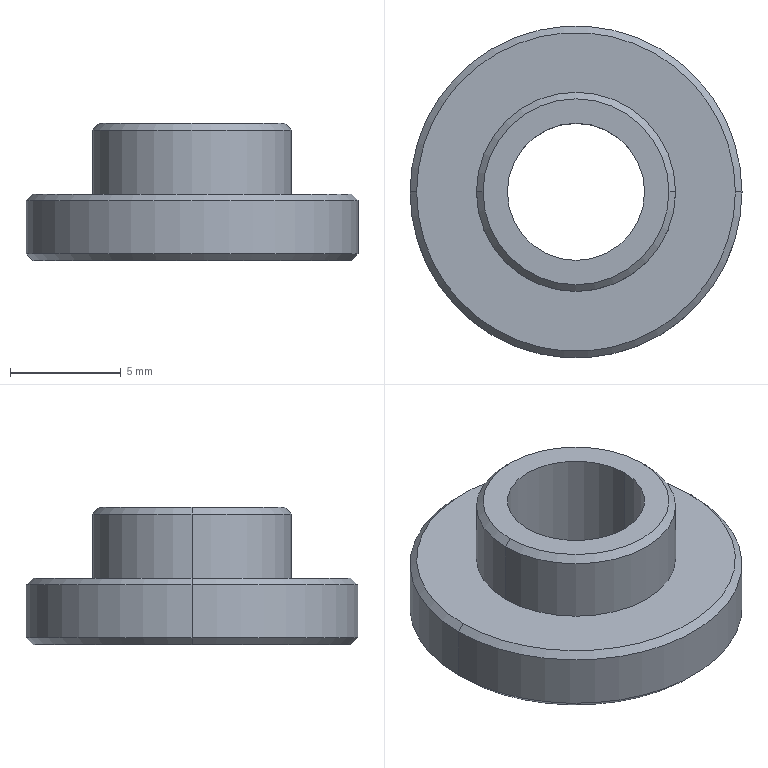Part | STEP file | Sprocket spacer | 1 solid | 15 faces | box 15 x 15 x 6.2 mm | volume 541.108 mm3 | cone 6 | cylinder 6 | plane 3 | commonest cylinder face diameters 6.2 x2 9 x2 15 x2
STEP:
#1=CARTESIAN_POINT('',(0.,0.,0.));
#2=DIRECTION('',(0.,0.,1.));
#3=DIRECTION('',(1.,0.,0.));
#4=AXIS2_PLACEMENT_3D('',#1,#2,#3);
#5=CARTESIAN_POINT('',(-7.2,0.,0.));
#6=VERTEX_POINT('',#5);
#7=CARTESIAN_POINT('',(7.2,0.,0.));
#8=VERTEX_POINT('',#7);
#9=CARTESIAN_POINT('',(0.,0.,0.));
#10=DIRECTION('',(0.,0.,-1.));
#11=DIRECTION('',(1.,0.,0.));
#12=AXIS2_PLACEMENT_3D('',#9,#10,#11);
#13=CIRCLE('',#12,7.2);
#14=CARTESIAN_POINT('',(0.,0.,0.));
#15=DIRECTION('',(0.,0.,1.));
#16=DIRECTION('',(1.,0.,0.));
#17=AXIS2_PLACEMENT_3D('',#14,#15,#16);
#18=CONICAL_SURFACE('',#17,7.2,0.7854);
#19=CARTESIAN_POINT('',(6.283,0.));
#20=DIRECTION('',(-1.,0.));
#21=VECTOR('',#20,1.);
#22=LINE('',#19,#21);
#23=(GEOMETRIC_REPRESENTATION_CONTEXT(2)PARAMETRIC_REPRESENTATION_CONTEXT()REPRESENTATION_CONTEXT('',''));
#24=DEFINITIONAL_REPRESENTATION('',(#22),#23);
#25=PCURVE('',#18,#24);
#26=CARTESIAN_POINT('',(0.,0.,0.));
#27=DIRECTION('',(0.,0.,1.));
#28=DIRECTION('',(1.,0.,0.));
#29=AXIS2_PLACEMENT_3D('',#26,#27,#28);
#30=PLANE('',#29);
#31=CARTESIAN_POINT('',(7.2,0.));
#32=CARTESIAN_POINT('',(7.2,-12.471));
#33=CARTESIAN_POINT('',(-3.6,-6.235));
#34=CARTESIAN_POINT('',(-14.4,0.));
#35=CARTESIAN_POINT('',(-3.6,6.235));
#36=CARTESIAN_POINT('',(7.2,12.471));
#37=CARTESIAN_POINT('',(7.2,0.));
#38=(BOUNDED_CURVE()B_SPLINE_CURVE(2,(#31,#32,#33,#34,#35,#36,#37),.UNSPECIFIED.,.T.,.F.)B_SPLINE_CURVE_WITH_KNOTS((1,2,2,2,2,1),(-2.094,0.,2.094,4.189,6.283,8.378),.UNSPECIFIED.)CURVE()GEOMETRIC_REPRESENTATION_ITEM()RATIONAL_B_SPLINE_CURVE((1.,0.5,1.,0.5,1.,0.5,1.))REPRESENTATION_ITEM(''));
#39=(GEOMETRIC_REPRESENTATION_CONTEXT(2)PARAMETRIC_REPRESENTATION_CONTEXT()REPRESENTATION_CONTEXT('',''));
#40=DEFINITIONAL_REPRESENTATION('',(#38),#39);
#41=PCURVE('',#30,#40);
#42=SURFACE_CURVE('',#13,(#25,#41),.PCURVE_S1.);
#43=EDGE_CURVE('',#6,#8,#42,.T.);
#44=ORIENTED_EDGE('',*,*,#43,.F.);
#45=CARTESIAN_POINT('',(-7.5,0.,0.3));
#46=VERTEX_POINT('',#45);
#47=CARTESIAN_POINT('',(-7.2,0.,0.));
#48=DIRECTION('',(-0.7071,0.,0.7071));
#49=VECTOR('',#48,1.);
#50=LINE('',#47,#49);
#51=CARTESIAN_POINT('',(3.142,0.));
#52=DIRECTION('',(0.,1.));
#53=VECTOR('',#52,1.);
#54=LINE('',#51,#53);
#55=(GEOMETRIC_REPRESENTATION_CONTEXT(2)PARAMETRIC_REPRESENTATION_CONTEXT()REPRESENTATION_CONTEXT('',''));
#56=DEFINITIONAL_REPRESENTATION('',(#54),#55);
#57=PCURVE('',#18,#56);
#58=CARTESIAN_POINT('',(0.,0.,0.));
#59=DIRECTION('',(0.,0.,1.));
#60=DIRECTION('',(1.,0.,0.));
#61=AXIS2_PLACEMENT_3D('',#58,#59,#60);
#62=CONICAL_SURFACE('',#61,7.2,0.7854);
#63=CARTESIAN_POINT('',(3.142,0.));
#64=DIRECTION('',(0.,1.));
#65=VECTOR('',#64,1.);
#66=LINE('',#63,#65);
#67=(GEOMETRIC_REPRESENTATION_CONTEXT(2)PARAMETRIC_REPRESENTATION_CONTEXT()REPRESENTATION_CONTEXT('',''));
#68=DEFINITIONAL_REPRESENTATION('',(#66),#67);
#69=PCURVE('',#62,#68);
#70=SURFACE_CURVE('',#50,(#57,#69),.PCURVE_S1.);
#71=EDGE_CURVE('',#6,#46,#70,.T.);
#72=ORIENTED_EDGE('',*,*,#71,.T.);
#73=CARTESIAN_POINT('',(7.5,0.,0.3));
#74=VERTEX_POINT('',#73);
#75=CARTESIAN_POINT('',(0.,0.,0.3));
#76=DIRECTION('',(0.,0.,1.));
#77=DIRECTION('',(1.,0.,0.));
#78=AXIS2_PLACEMENT_3D('',#75,#76,#77);
#79=CIRCLE('',#78,7.5);
#80=CARTESIAN_POINT('',(0.,0.3));
#81=DIRECTION('',(1.,0.));
#82=VECTOR('',#81,1.);
#83=LINE('',#80,#82);
#84=(GEOMETRIC_REPRESENTATION_CONTEXT(2)PARAMETRIC_REPRESENTATION_CONTEXT()REPRESENTATION_CONTEXT('',''));
#85=DEFINITIONAL_REPRESENTATION('',(#83),#84);
#86=PCURVE('',#18,#85);
#87=CARTESIAN_POINT('',(0.,0.,3.));
#88=DIRECTION('',(0.,0.,-1.));
#89=DIRECTION('',(-1.,0.,0.));
#90=AXIS2_PLACEMENT_3D('',#87,#88,#89);
#91=CYLINDRICAL_SURFACE('',#90,7.5);
#92=CARTESIAN_POINT('',(3.142,2.7));
#93=DIRECTION('',(-1.,0.));
#94=VECTOR('',#93,1.);
#95=LINE('',#92,#94);
#96=(GEOMETRIC_REPRESENTATION_CONTEXT(2)PARAMETRIC_REPRESENTATION_CONTEXT()REPRESENTATION_CONTEXT('',''));
#97=DEFINITIONAL_REPRESENTATION('',(#95),#96);
#98=PCURVE('',#91,#97);
#99=SURFACE_CURVE('',#79,(#86,#98),.PCURVE_S1.);
#100=EDGE_CURVE('',#74,#46,#99,.T.);
#101=ORIENTED_EDGE('',*,*,#100,.F.);
#102=CARTESIAN_POINT('',(7.2,0.,0.));
#103=DIRECTION('',(0.7071,0.,0.7071));
#104=VECTOR('',#103,1.);
#105=LINE('',#102,#104);
#106=CARTESIAN_POINT('',(0.,0.));
#107=DIRECTION('',(0.,1.));
#108=VECTOR('',#107,1.);
#109=LINE('',#106,#108);
#110=(GEOMETRIC_REPRESENTATION_CONTEXT(2)PARAMETRIC_REPRESENTATION_CONTEXT()REPRESENTATION_CONTEXT('',''));
#111=DEFINITIONAL_REPRESENTATION('',(#109),#110);
#112=PCURVE('',#18,#111);
#113=CARTESIAN_POINT('',(6.283,0.));
#114=DIRECTION('',(0.,1.));
#115=VECTOR('',#114,1.);
#116=LINE('',#113,#115);
#117=(GEOMETRIC_REPRESENTATION_CONTEXT(2)PARAMETRIC_REPRESENTATION_CONTEXT()REPRESENTATION_CONTEXT('',''));
#118=DEFINITIONAL_REPRESENTATION('',(#116),#117);
#119=PCURVE('',#62,#118);
#120=SURFACE_CURVE('',#105,(#112,#119),.PCURVE_S1.);
#121=EDGE_CURVE('',#8,#74,#120,.T.);
#122=ORIENTED_EDGE('',*,*,#121,.F.);
#123=EDGE_LOOP('',(#44,#72,#101,#122));
#124=FACE_BOUND('',#123,.T.);
#125=ADVANCED_FACE('',(#124),#18,.T.);
#126=CARTESIAN_POINT('',(7.2,0.,3.));
#127=VERTEX_POINT('',#126);
#128=CARTESIAN_POINT('',(-7.2,0.,3.));
#129=VERTEX_POINT('',#128);
#130=CARTESIAN_POINT('',(0.,0.,3.));
#131=DIRECTION('',(0.,0.,1.));
#132=DIRECTION('',(-1.,0.,0.));
#133=AXIS2_PLACEMENT_3D('',#130,#131,#132);
#134=CIRCLE('',#133,7.2);
#135=CARTESIAN_POINT('',(0.,0.,2.7));
#136=DIRECTION('',(0.,0.,-1.));
#137=DIRECTION('',(-1.,0.,0.));
#138=AXIS2_PLACEMENT_3D('',#135,#136,#137);
#139=CONICAL_SURFACE('',#138,7.5,0.7854);
#140=CARTESIAN_POINT('',(6.283,-0.3));
#141=DIRECTION('',(-1.,0.));
#142=VECTOR('',#141,1.);
#143=LINE('',#140,#142);
#144=(GEOMETRIC_REPRESENTATION_CONTEXT(2)PARAMETRIC_REPRESENTATION_CONTEXT()REPRESENTATION_CONTEXT('',''));
#145=DEFINITIONAL_REPRESENTATION('',(#143),#144);
#146=PCURVE('',#139,#145);
#147=CARTESIAN_POINT('',(0.,0.,3.));
#148=DIRECTION('',(0.,0.,-1.));
#149=DIRECTION('',(-1.,0.,0.));
#150=AXIS2_PLACEMENT_3D('',#147,#148,#149);
#151=PLANE('',#150);
#152=CARTESIAN_POINT('',(7.2,0.));
#153=CARTESIAN_POINT('',(7.2,-12.471));
#154=CARTESIAN_POINT('',(-3.6,-6.235));
#155=CARTESIAN_POINT('',(-14.4,0.));
#156=CARTESIAN_POINT('',(-3.6,6.235));
#157=CARTESIAN_POINT('',(7.2,12.471));
#158=CARTESIAN_POINT('',(7.2,0.));
#159=(BOUNDED_CURVE()B_SPLINE_CURVE(2,(#152,#153,#154,#155,#156,#157,#158),.UNSPECIFIED.,.T.,.F.)B_SPLINE_CURVE_WITH_KNOTS((1,2,2,2,2,1),(-2.094,0.,2.094,4.189,6.283,8.378),.UNSPECIFIED.)CURVE()GEOMETRIC_REPRESENTATION_ITEM()RATIONAL_B_SPLINE_CURVE((1.,0.5,1.,0.5,1.,0.5,1.))REPRESENTATION_ITEM(''));
#160=(GEOMETRIC_REPRESENTATION_CONTEXT(2)PARAMETRIC_REPRESENTATION_CONTEXT()REPRESENTATION_CONTEXT('',''));
#161=DEFINITIONAL_REPRESENTATION('',(#159),#160);
#162=PCURVE('',#151,#161);
#163=SURFACE_CURVE('',#134,(#146,#162),.PCURVE_S1.);
#164=EDGE_CURVE('',#127,#129,#163,.T.);
#165=ORIENTED_EDGE('',*,*,#164,.F.);
#166=CARTESIAN_POINT('',(7.5,0.,2.7));
#167=VERTEX_POINT('',#166);
#168=CARTESIAN_POINT('',(7.5,0.,2.7));
#169=DIRECTION('',(0.7071,0.,-0.7071));
#170=VECTOR('',#169,1.);
#171=LINE('',#168,#170);
#172=CARTESIAN_POINT('',(3.142,0.));
#173=DIRECTION('',(0.,1.));
#174=VECTOR('',#173,1.);
#175=LINE('',#172,#174);
#176=(GEOMETRIC_REPRESENTATION_CONTEXT(2)PARAMETRIC_REPRESENTATION_CONTEXT()REPRESENTATION_CONTEXT('',''));
#177=DEFINITIONAL_REPRESENTATION('',(#175),#176);
#178=PCURVE('',#139,#177);
#179=CARTESIAN_POINT('',(0.,0.,2.7));
#180=DIRECTION('',(0.,0.,-1.));
#181=DIRECTION('',(-1.,0.,0.));
#182=AXIS2_PLACEMENT_3D('',#179,#180,#181);
#183=CONICAL_SURFACE('',#182,7.5,0.7854);
#184=CARTESIAN_POINT('',(3.142,0.));
#185=DIRECTION('',(0.,1.));
#186=VECTOR('',#185,1.);
#187=LINE('',#184,#186);
#188=(GEOMETRIC_REPRESENTATION_CONTEXT(2)PARAMETRIC_REPRESENTATION_CONTEXT()REPRESENTATION_CONTEXT('',''));
#189=DEFINITIONAL_REPRESENTATION('',(#187),#188);
#190=PCURVE('',#183,#189);
#191=SURFACE_CURVE('',#171,(#178,#190),.PCURVE_S1.);
#192=EDGE_CURVE('',#127,#167,#191,.T.);
#193=ORIENTED_EDGE('',*,*,#192,.T.);
#194=CARTESIAN_POINT('',(-7.5,0.,2.7));
#195=VERTEX_POINT('',#194);
#196=CARTESIAN_POINT('',(0.,0.,2.7));
#197=DIRECTION('',(0.,0.,-1.));
#198=DIRECTION('',(-1.,0.,0.));
#199=AXIS2_PLACEMENT_3D('',#196,#197,#198);
#200=CIRCLE('',#199,7.5);
#201=CARTESIAN_POINT('',(0.,0.));
#202=DIRECTION('',(1.,0.));
#203=VECTOR('',#202,1.);
#204=LINE('',#201,#203);
#205=(GEOMETRIC_REPRESENTATION_CONTEXT(2)PARAMETRIC_REPRESENTATION_CONTEXT()REPRESENTATION_CONTEXT('',''));
#206=DEFINITIONAL_REPRESENTATION('',(#204),#205);
#207=PCURVE('',#139,#206);
#208=CARTESIAN_POINT('',(0.,0.3));
#209=DIRECTION('',(1.,0.));
#210=VECTOR('',#209,1.);
#211=LINE('',#208,#210);
#212=(GEOMETRIC_REPRESENTATION_CONTEXT(2)PARAMETRIC_REPRESENTATION_CONTEXT()REPRESENTATION_CONTEXT('',''));
#213=DEFINITIONAL_REPRESENTATION('',(#211),#212);
#214=PCURVE('',#91,#213);
#215=SURFACE_CURVE('',#200,(#207,#214),.PCURVE_S1.);
#216=EDGE_CURVE('',#195,#167,#215,.T.);
#217=ORIENTED_EDGE('',*,*,#216,.F.);
#218=CARTESIAN_POINT('',(-7.5,0.,2.7));
#219=DIRECTION('',(-0.7071,0.,-0.7071));
#220=VECTOR('',#219,1.);
#221=LINE('',#218,#220);
#222=CARTESIAN_POINT('',(0.,0.));
#223=DIRECTION('',(0.,1.));
#224=VECTOR('',#223,1.);
#225=LINE('',#222,#224);
#226=(GEOMETRIC_REPRESENTATION_CONTEXT(2)PARAMETRIC_REPRESENTATION_CONTEXT()REPRESENTATION_CONTEXT('',''));
#227=DEFINITIONAL_REPRESENTATION('',(#225),#226);
#228=PCURVE('',#139,#227);
#229=CARTESIAN_POINT('',(6.283,0.));
#230=DIRECTION('',(0.,1.));
#231=VECTOR('',#230,1.);
#232=LINE('',#229,#231);
#233=(GEOMETRIC_REPRESENTATION_CONTEXT(2)PARAMETRIC_REPRESENTATION_CONTEXT()REPRESENTATION_CONTEXT('',''));
#234=DEFINITIONAL_REPRESENTATION('',(#232),#233);
#235=PCURVE('',#183,#234);
#236=SURFACE_CURVE('',#221,(#228,#235),.PCURVE_S1.);
#237=EDGE_CURVE('',#129,#195,#236,.T.);
#238=ORIENTED_EDGE('',*,*,#237,.F.);
#239=EDGE_LOOP('',(#165,#193,#217,#238));
#240=FACE_BOUND('',#239,.T.);
#241=ADVANCED_FACE('',(#240),#139,.T.);
#242=CARTESIAN_POINT('',(4.2,0.,6.2));
#243=VERTEX_POINT('',#242);
#244=CARTESIAN_POINT('',(-4.2,0.,6.2));
#245=VERTEX_POINT('',#244);
#246=CARTESIAN_POINT('',(0.,0.,6.2));
#247=DIRECTION('',(0.,0.,1.));
#248=DIRECTION('',(1.,0.,0.));
#249=AXIS2_PLACEMENT_3D('',#246,#247,#248);
#250=CIRCLE('',#249,4.2);
#251=CARTESIAN_POINT('',(0.,0.,6.2));
#252=DIRECTION('',(0.,0.,-1.));
#253=DIRECTION('',(-1.,0.,0.));
#254=AXIS2_PLACEMENT_3D('',#251,#252,#253);
#255=CONICAL_SURFACE('',#254,4.2,0.7854);
#256=CARTESIAN_POINT('',(3.142,0.));
#257=DIRECTION('',(-1.,0.));
#258=VECTOR('',#257,1.);
#259=LINE('',#256,#258);
#260=(GEOMETRIC_REPRESENTATION_CONTEXT(2)PARAMETRIC_REPRESENTATION_CONTEXT()REPRESENTATION_CONTEXT('',''));
#261=DEFINITIONAL_REPRESENTATION('',(#259),#260);
#262=PCURVE('',#255,#261);
#263=CARTESIAN_POINT('',(0.,0.,6.2));
#264=DIRECTION('',(0.,0.,1.));
#265=DIRECTION('',(1.,0.,0.));
#266=AXIS2_PLACEMENT_3D('',#263,#264,#265);
#267=PLANE('',#266);
#268=CARTESIAN_POINT('',(0.,0.));
#269=DIRECTION('',(1.,0.));
#270=AXIS2_PLACEMENT_2D('',#268,#269);
#271=CIRCLE('',#270,4.2);
#272=(GEOMETRIC_REPRESENTATION_CONTEXT(2)PARAMETRIC_REPRESENTATION_CONTEXT()REPRESENTATION_CONTEXT('',''));
#273=DEFINITIONAL_REPRESENTATION('',(#271),#272);
#274=PCURVE('',#267,#273);
#275=SURFACE_CURVE('',#250,(#262,#274),.PCURVE_S1.);
#276=EDGE_CURVE('',#243,#245,#275,.T.);
#277=ORIENTED_EDGE('',*,*,#276,.F.);
#278=CARTESIAN_POINT('',(4.5,0.,5.9));
#279=VERTEX_POINT('',#278);
#280=CARTESIAN_POINT('',(4.2,0.,6.2));
#281=DIRECTION('',(0.7071,0.,-0.7071));
#282=VECTOR('',#281,1.);
#283=LINE('',#280,#282);
#284=CARTESIAN_POINT('',(3.142,0.));
#285=DIRECTION('',(0.,1.));
#286=VECTOR('',#285,1.);
#287=LINE('',#284,#286);
#288=(GEOMETRIC_REPRESENTATION_CONTEXT(2)PARAMETRIC_REPRESENTATION_CONTEXT()REPRESENTATION_CONTEXT('',''));
#289=DEFINITIONAL_REPRESENTATION('',(#287),#288);
#290=PCURVE('',#255,#289);
#291=CARTESIAN_POINT('',(0.,0.,6.2));
#292=DIRECTION('',(0.,0.,-1.));
#293=DIRECTION('',(-1.,0.,0.));
#294=AXIS2_PLACEMENT_3D('',#291,#292,#293);
#295=CONICAL_SURFACE('',#294,4.2,0.7854);
#296=CARTESIAN_POINT('',(3.142,0.));
#297=DIRECTION('',(0.,1.));
#298=VECTOR('',#297,1.);
#299=LINE('',#296,#298);
#300=(GEOMETRIC_REPRESENTATION_CONTEXT(2)PARAMETRIC_REPRESENTATION_CONTEXT()REPRESENTATION_CONTEXT('',''));
#301=DEFINITIONAL_REPRESENTATION('',(#299),#300);
#302=PCURVE('',#295,#301);
#303=SURFACE_CURVE('',#283,(#290,#302),.PCURVE_S1.);
#304=EDGE_CURVE('',#243,#279,#303,.T.);
#305=ORIENTED_EDGE('',*,*,#304,.T.);
#306=CARTESIAN_POINT('',(-4.5,0.,5.9));
#307=VERTEX_POINT('',#306);
#308=CARTESIAN_POINT('',(0.,0.,5.9));
#309=DIRECTION('',(0.,0.,-1.));
#310=DIRECTION('',(1.,0.,0.));
#311=AXIS2_PLACEMENT_3D('',#308,#309,#310);
#312=CIRCLE('',#311,4.5);
#313=CARTESIAN_POINT('',(-3.142,0.3));
#314=DIRECTION('',(1.,0.));
#315=VECTOR('',#314,1.);
#316=LINE('',#313,#315);
#317=(GEOMETRIC_REPRESENTATION_CONTEXT(2)PARAMETRIC_REPRESENTATION_CONTEXT()REPRESENTATION_CONTEXT('',''));
#318=DEFINITIONAL_REPRESENTATION('',(#316),#317);
#319=PCURVE('',#255,#318);
#320=CARTESIAN_POINT('',(0.,0.,6.2));
#321=DIRECTION('',(0.,0.,-1.));
#322=DIRECTION('',(-1.,0.,0.));
#323=AXIS2_PLACEMENT_3D('',#320,#321,#322);
#324=CYLINDRICAL_SURFACE('',#323,4.5);
#325=CARTESIAN_POINT('',(-3.142,0.3));
#326=DIRECTION('',(1.,0.));
#327=VECTOR('',#326,1.);
#328=LINE('',#325,#327);
#329=(GEOMETRIC_REPRESENTATION_CONTEXT(2)PARAMETRIC_REPRESENTATION_CONTEXT()REPRESENTATION_CONTEXT('',''));
#330=DEFINITIONAL_REPRESENTATION('',(#328),#329);
#331=PCURVE('',#324,#330);
#332=SURFACE_CURVE('',#312,(#319,#331),.PCURVE_S1.);
#333=EDGE_CURVE('',#307,#279,#332,.T.);
#334=ORIENTED_EDGE('',*,*,#333,.F.);
#335=CARTESIAN_POINT('',(-4.2,0.,6.2));
#336=DIRECTION('',(-0.7071,0.,-0.7071));
#337=VECTOR('',#336,1.);
#338=LINE('',#335,#337);
#339=CARTESIAN_POINT('',(0.,0.));
#340=DIRECTION('',(0.,1.));
#341=VECTOR('',#340,1.);
#342=LINE('',#339,#341);
#343=(GEOMETRIC_REPRESENTATION_CONTEXT(2)PARAMETRIC_REPRESENTATION_CONTEXT()REPRESENTATION_CONTEXT('',''));
#344=DEFINITIONAL_REPRESENTATION('',(#342),#343);
#345=PCURVE('',#255,#344);
#346=CARTESIAN_POINT('',(6.283,0.));
#347=DIRECTION('',(0.,1.));
#348=VECTOR('',#347,1.);
#349=LINE('',#346,#348);
#350=(GEOMETRIC_REPRESENTATION_CONTEXT(2)PARAMETRIC_REPRESENTATION_CONTEXT()REPRESENTATION_CONTEXT('',''));
#351=DEFINITIONAL_REPRESENTATION('',(#349),#350);
#352=PCURVE('',#295,#351);
#353=SURFACE_CURVE('',#338,(#345,#352),.PCURVE_S1.);
#354=EDGE_CURVE('',#245,#307,#353,.T.);
#355=ORIENTED_EDGE('',*,*,#354,.F.);
#356=EDGE_LOOP('',(#277,#305,#334,#355));
#357=FACE_BOUND('',#356,.T.);
#358=ADVANCED_FACE('',(#357),#255,.T.);
#359=ORIENTED_EDGE('',*,*,#216,.T.);
#360=CARTESIAN_POINT('',(7.5,0.,3.));
#361=DIRECTION('',(0.,0.,-1.));
#362=VECTOR('',#361,1.);
#363=LINE('',#360,#362);
#364=CARTESIAN_POINT('',(3.142,0.));
#365=DIRECTION('',(0.,1.));
#366=VECTOR('',#365,1.);
#367=LINE('',#364,#366);
#368=(GEOMETRIC_REPRESENTATION_CONTEXT(2)PARAMETRIC_REPRESENTATION_CONTEXT()REPRESENTATION_CONTEXT('',''));
#369=DEFINITIONAL_REPRESENTATION('',(#367),#368);
#370=PCURVE('',#91,#369);
#371=CARTESIAN_POINT('',(0.,0.,3.));
#372=DIRECTION('',(0.,0.,-1.));
#373=DIRECTION('',(-1.,0.,0.));
#374=AXIS2_PLACEMENT_3D('',#371,#372,#373);
#375=CYLINDRICAL_SURFACE('',#374,7.5);
#376=CARTESIAN_POINT('',(3.142,0.));
#377=DIRECTION('',(0.,1.));
#378=VECTOR('',#377,1.);
#379=LINE('',#376,#378);
#380=(GEOMETRIC_REPRESENTATION_CONTEXT(2)PARAMETRIC_REPRESENTATION_CONTEXT()REPRESENTATION_CONTEXT('',''));
#381=DEFINITIONAL_REPRESENTATION('',(#379),#380);
#382=PCURVE('',#375,#381);
#383=SURFACE_CURVE('',#363,(#370,#382),.PCURVE_S1.);
#384=EDGE_CURVE('',#167,#74,#383,.T.);
#385=ORIENTED_EDGE('',*,*,#384,.T.);
#386=ORIENTED_EDGE('',*,*,#100,.T.);
#387=CARTESIAN_POINT('',(-7.5,0.,3.));
#388=DIRECTION('',(0.,0.,-1.));
#389=VECTOR('',#388,1.);
#390=LINE('',#387,#389);
#391=CARTESIAN_POINT('',(0.,0.));
#392=DIRECTION('',(0.,1.));
#393=VECTOR('',#392,1.);
#394=LINE('',#391,#393);
#395=(GEOMETRIC_REPRESENTATION_CONTEXT(2)PARAMETRIC_REPRESENTATION_CONTEXT()REPRESENTATION_CONTEXT('',''));
#396=DEFINITIONAL_REPRESENTATION('',(#394),#395);
#397=PCURVE('',#91,#396);
#398=CARTESIAN_POINT('',(6.283,0.));
#399=DIRECTION('',(0.,1.));
#400=VECTOR('',#399,1.);
#401=LINE('',#398,#400);
#402=(GEOMETRIC_REPRESENTATION_CONTEXT(2)PARAMETRIC_REPRESENTATION_CONTEXT()REPRESENTATION_CONTEXT('',''));
#403=DEFINITIONAL_REPRESENTATION('',(#401),#402);
#404=PCURVE('',#375,#403);
#405=SURFACE_CURVE('',#390,(#397,#404),.PCURVE_S1.);
#406=EDGE_CURVE('',#195,#46,#405,.T.);
#407=ORIENTED_EDGE('',*,*,#406,.F.);
#408=EDGE_LOOP('',(#359,#385,#386,#407));
#409=FACE_BOUND('',#408,.T.);
#410=ADVANCED_FACE('',(#409),#91,.T.);
#411=CARTESIAN_POINT('',(-3.1,0.,6.2));
#412=VERTEX_POINT('',#411);
#413=CARTESIAN_POINT('',(-3.1,0.,0.));
#414=VERTEX_POINT('',#413);
#415=CARTESIAN_POINT('',(-3.1,0.,6.2));
#416=DIRECTION('',(0.,0.,-1.));
#417=VECTOR('',#416,1.);
#418=LINE('',#415,#417);
#419=CARTESIAN_POINT('',(0.,0.,6.2));
#420=DIRECTION('',(0.,0.,-1.));
#421=DIRECTION('',(-1.,0.,0.));
#422=AXIS2_PLACEMENT_3D('',#419,#420,#421);
#423=CYLINDRICAL_SURFACE('',#422,3.1);
#424=CARTESIAN_POINT('',(6.283,0.));
#425=DIRECTION('',(0.,1.));
#426=VECTOR('',#425,1.);
#427=LINE('',#424,#426);
#428=(GEOMETRIC_REPRESENTATION_CONTEXT(2)PARAMETRIC_REPRESENTATION_CONTEXT()REPRESENTATION_CONTEXT('',''));
#429=DEFINITIONAL_REPRESENTATION('',(#427),#428);
#430=PCURVE('',#423,#429);
#431=CARTESIAN_POINT('',(0.,0.,6.2));
#432=DIRECTION('',(0.,0.,-1.));
#433=DIRECTION('',(-1.,0.,0.));
#434=AXIS2_PLACEMENT_3D('',#431,#432,#433);
#435=CYLINDRICAL_SURFACE('',#434,3.1);
#436=CARTESIAN_POINT('',(0.,0.));
#437=DIRECTION('',(0.,1.));
#438=VECTOR('',#437,1.);
#439=LINE('',#436,#438);
#440=(GEOMETRIC_REPRESENTATION_CONTEXT(2)PARAMETRIC_REPRESENTATION_CONTEXT()REPRESENTATION_CONTEXT('',''));
#441=DEFINITIONAL_REPRESENTATION('',(#439),#440);
#442=PCURVE('',#435,#441);
#443=SURFACE_CURVE('',#418,(#430,#442),.PCURVE_S1.);
#444=EDGE_CURVE('',#412,#414,#443,.T.);
#445=ORIENTED_EDGE('',*,*,#444,.T.);
#446=CARTESIAN_POINT('',(3.1,0.,0.));
#447=VERTEX_POINT('',#446);
#448=CARTESIAN_POINT('',(0.,0.,0.));
#449=DIRECTION('',(0.,0.,1.));
#450=DIRECTION('',(1.,0.,0.));
#451=AXIS2_PLACEMENT_3D('',#448,#449,#450);
#452=CIRCLE('',#451,3.1);
#453=CARTESIAN_POINT('',(9.425,6.2));
#454=DIRECTION('',(-1.,0.));
#455=VECTOR('',#454,1.);
#456=LINE('',#453,#455);
#457=(GEOMETRIC_REPRESENTATION_CONTEXT(2)PARAMETRIC_REPRESENTATION_CONTEXT()REPRESENTATION_CONTEXT('',''));
#458=DEFINITIONAL_REPRESENTATION('',(#456),#457);
#459=PCURVE('',#423,#458);
#460=CARTESIAN_POINT('',(0.,0.));
#461=DIRECTION('',(1.,0.));
#462=AXIS2_PLACEMENT_2D('',#460,#461);
#463=CIRCLE('',#462,3.1);
#464=(GEOMETRIC_REPRESENTATION_CONTEXT(2)PARAMETRIC_REPRESENTATION_CONTEXT()REPRESENTATION_CONTEXT('',''));
#465=DEFINITIONAL_REPRESENTATION('',(#463),#464);
#466=PCURVE('',#30,#465);
#467=SURFACE_CURVE('',#452,(#459,#466),.PCURVE_S1.);
#468=EDGE_CURVE('',#414,#447,#467,.T.);
#469=ORIENTED_EDGE('',*,*,#468,.T.);
#470=CARTESIAN_POINT('',(3.1,0.,6.2));
#471=VERTEX_POINT('',#470);
#472=CARTESIAN_POINT('',(3.1,0.,6.2));
#473=DIRECTION('',(0.,0.,-1.));
#474=VECTOR('',#473,1.);
#475=LINE('',#472,#474);
#476=CARTESIAN_POINT('',(3.142,0.));
#477=DIRECTION('',(0.,1.));
#478=VECTOR('',#477,1.);
#479=LINE('',#476,#478);
#480=(GEOMETRIC_REPRESENTATION_CONTEXT(2)PARAMETRIC_REPRESENTATION_CONTEXT()REPRESENTATION_CONTEXT('',''));
#481=DEFINITIONAL_REPRESENTATION('',(#479),#480);
#482=PCURVE('',#423,#481);
#483=CARTESIAN_POINT('',(3.142,0.));
#484=DIRECTION('',(0.,1.));
#485=VECTOR('',#484,1.);
#486=LINE('',#483,#485);
#487=(GEOMETRIC_REPRESENTATION_CONTEXT(2)PARAMETRIC_REPRESENTATION_CONTEXT()REPRESENTATION_CONTEXT('',''));
#488=DEFINITIONAL_REPRESENTATION('',(#486),#487);
#489=PCURVE('',#435,#488);
#490=SURFACE_CURVE('',#475,(#482,#489),.PCURVE_S1.);
#491=EDGE_CURVE('',#471,#447,#490,.T.);
#492=ORIENTED_EDGE('',*,*,#491,.F.);
#493=CARTESIAN_POINT('',(0.,0.,6.2));
#494=DIRECTION('',(0.,0.,1.));
#495=DIRECTION('',(1.,0.,0.));
#496=AXIS2_PLACEMENT_3D('',#493,#494,#495);
#497=CIRCLE('',#496,3.1);
#498=CARTESIAN_POINT('',(9.425,0.));
#499=DIRECTION('',(-1.,0.));
#500=VECTOR('',#499,1.);
#501=LINE('',#498,#500);
#502=(GEOMETRIC_REPRESENTATION_CONTEXT(2)PARAMETRIC_REPRESENTATION_CONTEXT()REPRESENTATION_CONTEXT('',''));
#503=DEFINITIONAL_REPRESENTATION('',(#501),#502);
#504=PCURVE('',#423,#503);
#505=CARTESIAN_POINT('',(0.,0.));
#506=DIRECTION('',(1.,0.));
#507=AXIS2_PLACEMENT_2D('',#505,#506);
#508=CIRCLE('',#507,3.1);
#509=(GEOMETRIC_REPRESENTATION_CONTEXT(2)PARAMETRIC_REPRESENTATION_CONTEXT()REPRESENTATION_CONTEXT('',''));
#510=DEFINITIONAL_REPRESENTATION('',(#508),#509);
#511=PCURVE('',#267,#510);
#512=SURFACE_CURVE('',#497,(#504,#511),.PCURVE_S1.);
#513=EDGE_CURVE('',#412,#471,#512,.T.);
#514=ORIENTED_EDGE('',*,*,#513,.F.);
#515=EDGE_LOOP('',(#445,#469,#492,#514));
#516=FACE_BOUND('',#515,.F.);
#517=ADVANCED_FACE('',(#516),#423,.F.);
#518=ORIENTED_EDGE('',*,*,#333,.T.);
#519=CARTESIAN_POINT('',(4.5,0.,3.));
#520=VERTEX_POINT('',#519);
#521=CARTESIAN_POINT('',(4.5,0.,6.2));
#522=DIRECTION('',(0.,0.,-1.));
#523=VECTOR('',#522,1.);
#524=LINE('',#521,#523);
#525=CARTESIAN_POINT('',(3.142,0.));
#526=DIRECTION('',(0.,1.));
#527=VECTOR('',#526,1.);
#528=LINE('',#525,#527);
#529=(GEOMETRIC_REPRESENTATION_CONTEXT(2)PARAMETRIC_REPRESENTATION_CONTEXT()REPRESENTATION_CONTEXT('',''));
#530=DEFINITIONAL_REPRESENTATION('',(#528),#529);
#531=PCURVE('',#324,#530);
#532=CARTESIAN_POINT('',(0.,0.,6.2));
#533=DIRECTION('',(0.,0.,-1.));
#534=DIRECTION('',(-1.,0.,0.));
#535=AXIS2_PLACEMENT_3D('',#532,#533,#534);
#536=CYLINDRICAL_SURFACE('',#535,4.5);
#537=CARTESIAN_POINT('',(3.142,0.));
#538=DIRECTION('',(0.,1.));
#539=VECTOR('',#538,1.);
#540=LINE('',#537,#539);
#541=(GEOMETRIC_REPRESENTATION_CONTEXT(2)PARAMETRIC_REPRESENTATION_CONTEXT()REPRESENTATION_CONTEXT('',''));
#542=DEFINITIONAL_REPRESENTATION('',(#540),#541);
#543=PCURVE('',#536,#542);
#544=SURFACE_CURVE('',#524,(#531,#543),.PCURVE_S1.);
#545=EDGE_CURVE('',#279,#520,#544,.T.);
#546=ORIENTED_EDGE('',*,*,#545,.T.);
#547=CARTESIAN_POINT('',(-4.5,0.,3.));
#548=VERTEX_POINT('',#547);
#549=CARTESIAN_POINT('',(0.,0.,3.));
#550=DIRECTION('',(0.,0.,-1.));
#551=DIRECTION('',(-1.,0.,0.));
#552=AXIS2_PLACEMENT_3D('',#549,#550,#551);
#553=CIRCLE('',#552,4.5);
#554=CARTESIAN_POINT('',(0.,3.2));
#555=DIRECTION('',(1.,0.));
#556=VECTOR('',#555,1.);
#557=LINE('',#554,#556);
#558=(GEOMETRIC_REPRESENTATION_CONTEXT(2)PARAMETRIC_REPRESENTATION_CONTEXT()REPRESENTATION_CONTEXT('',''));
#559=DEFINITIONAL_REPRESENTATION('',(#557),#558);
#560=PCURVE('',#324,#559);
#561=CARTESIAN_POINT('',(0.,0.));
#562=DIRECTION('',(1.,0.));
#563=AXIS2_PLACEMENT_2D('',#561,#562);
#564=CIRCLE('',#563,4.5);
#565=(GEOMETRIC_REPRESENTATION_CONTEXT(2)PARAMETRIC_REPRESENTATION_CONTEXT()REPRESENTATION_CONTEXT('',''));
#566=DEFINITIONAL_REPRESENTATION('',(#564),#565);
#567=PCURVE('',#151,#566);
#568=SURFACE_CURVE('',#553,(#560,#567),.PCURVE_S1.);
#569=EDGE_CURVE('',#548,#520,#568,.T.);
#570=ORIENTED_EDGE('',*,*,#569,.F.);
#571=CARTESIAN_POINT('',(-4.5,0.,6.2));
#572=DIRECTION('',(0.,0.,-1.));
#573=VECTOR('',#572,1.);
#574=LINE('',#571,#573);
#575=CARTESIAN_POINT('',(0.,0.));
#576=DIRECTION('',(0.,1.));
#577=VECTOR('',#576,1.);
#578=LINE('',#575,#577);
#579=(GEOMETRIC_REPRESENTATION_CONTEXT(2)PARAMETRIC_REPRESENTATION_CONTEXT()REPRESENTATION_CONTEXT('',''));
#580=DEFINITIONAL_REPRESENTATION('',(#578),#579);
#581=PCURVE('',#324,#580);
#582=CARTESIAN_POINT('',(6.283,0.));
#583=DIRECTION('',(0.,1.));
#584=VECTOR('',#583,1.);
#585=LINE('',#582,#584);
#586=(GEOMETRIC_REPRESENTATION_CONTEXT(2)PARAMETRIC_REPRESENTATION_CONTEXT()REPRESENTATION_CONTEXT('',''));
#587=DEFINITIONAL_REPRESENTATION('',(#585),#586);
#588=PCURVE('',#536,#587);
#589=SURFACE_CURVE('',#574,(#581,#588),.PCURVE_S1.);
#590=EDGE_CURVE('',#307,#548,#589,.T.);
#591=ORIENTED_EDGE('',*,*,#590,.F.);
#592=EDGE_LOOP('',(#518,#546,#570,#591));
#593=FACE_BOUND('',#592,.T.);
#594=ADVANCED_FACE('',(#593),#324,.T.);
#595=ORIENTED_EDGE('',*,*,#545,.F.);
#596=CARTESIAN_POINT('',(0.,0.,5.9));
#597=DIRECTION('',(0.,0.,-1.));
#598=DIRECTION('',(1.,0.,0.));
#599=AXIS2_PLACEMENT_3D('',#596,#597,#598);
#600=CIRCLE('',#599,4.5);
#601=CARTESIAN_POINT('',(3.142,0.3));
#602=DIRECTION('',(1.,0.));
#603=VECTOR('',#602,1.);
#604=LINE('',#601,#603);
#605=(GEOMETRIC_REPRESENTATION_CONTEXT(2)PARAMETRIC_REPRESENTATION_CONTEXT()REPRESENTATION_CONTEXT('',''));
#606=DEFINITIONAL_REPRESENTATION('',(#604),#605);
#607=PCURVE('',#536,#606);
#608=CARTESIAN_POINT('',(3.142,0.3));
#609=DIRECTION('',(1.,0.));
#610=VECTOR('',#609,1.);
#611=LINE('',#608,#610);
#612=(GEOMETRIC_REPRESENTATION_CONTEXT(2)PARAMETRIC_REPRESENTATION_CONTEXT()REPRESENTATION_CONTEXT('',''));
#613=DEFINITIONAL_REPRESENTATION('',(#611),#612);
#614=PCURVE('',#295,#613);
#615=SURFACE_CURVE('',#600,(#607,#614),.PCURVE_S1.);
#616=EDGE_CURVE('',#279,#307,#615,.T.);
#617=ORIENTED_EDGE('',*,*,#616,.T.);
#618=ORIENTED_EDGE('',*,*,#590,.T.);
#619=CARTESIAN_POINT('',(0.,0.,3.));
#620=DIRECTION('',(0.,0.,-1.));
#621=DIRECTION('',(-1.,0.,0.));
#622=AXIS2_PLACEMENT_3D('',#619,#620,#621);
#623=CIRCLE('',#622,4.5);
#624=CARTESIAN_POINT('',(0.,3.2));
#625=DIRECTION('',(1.,0.));
#626=VECTOR('',#625,1.);
#627=LINE('',#624,#626);
#628=(GEOMETRIC_REPRESENTATION_CONTEXT(2)PARAMETRIC_REPRESENTATION_CONTEXT()REPRESENTATION_CONTEXT('',''));
#629=DEFINITIONAL_REPRESENTATION('',(#627),#628);
#630=PCURVE('',#536,#629);
#631=CARTESIAN_POINT('',(0.,0.));
#632=DIRECTION('',(1.,0.));
#633=AXIS2_PLACEMENT_2D('',#631,#632);
#634=CIRCLE('',#633,4.5);
#635=(GEOMETRIC_REPRESENTATION_CONTEXT(2)PARAMETRIC_REPRESENTATION_CONTEXT()REPRESENTATION_CONTEXT('',''));
#636=DEFINITIONAL_REPRESENTATION('',(#634),#635);
#637=PCURVE('',#151,#636);
#638=SURFACE_CURVE('',#623,(#630,#637),.PCURVE_S1.);
#639=EDGE_CURVE('',#520,#548,#638,.T.);
#640=ORIENTED_EDGE('',*,*,#639,.F.);
#641=EDGE_LOOP('',(#595,#617,#618,#640));
#642=FACE_BOUND('',#641,.T.);
#643=ADVANCED_FACE('',(#642),#536,.T.);
#644=CARTESIAN_POINT('',(0.,0.,6.2));
#645=DIRECTION('',(0.,0.,1.));
#646=DIRECTION('',(1.,0.,0.));
#647=AXIS2_PLACEMENT_3D('',#644,#645,#646);
#648=CIRCLE('',#647,4.2);
#649=CARTESIAN_POINT('',(0.,0.));
#650=DIRECTION('',(1.,0.));
#651=AXIS2_PLACEMENT_2D('',#649,#650);
#652=CIRCLE('',#651,4.2);
#653=(GEOMETRIC_REPRESENTATION_CONTEXT(2)PARAMETRIC_REPRESENTATION_CONTEXT()REPRESENTATION_CONTEXT('',''));
#654=DEFINITIONAL_REPRESENTATION('',(#652),#653);
#655=PCURVE('',#267,#654);
#656=CARTESIAN_POINT('',(9.425,0.));
#657=DIRECTION('',(-1.,0.));
#658=VECTOR('',#657,1.);
#659=LINE('',#656,#658);
#660=(GEOMETRIC_REPRESENTATION_CONTEXT(2)PARAMETRIC_REPRESENTATION_CONTEXT()REPRESENTATION_CONTEXT('',''));
#661=DEFINITIONAL_REPRESENTATION('',(#659),#660);
#662=PCURVE('',#295,#661);
#663=SURFACE_CURVE('',#648,(#655,#662),.PCURVE_S1.);
#664=EDGE_CURVE('',#245,#243,#663,.T.);
#665=ORIENTED_EDGE('',*,*,#664,.T.);
#666=ORIENTED_EDGE('',*,*,#276,.T.);
#667=EDGE_LOOP('',(#665,#666));
#668=FACE_BOUND('',#667,.T.);
#669=ORIENTED_EDGE('',*,*,#513,.F.);
#670=CARTESIAN_POINT('',(0.,0.,6.2));
#671=DIRECTION('',(0.,0.,1.));
#672=DIRECTION('',(1.,0.,0.));
#673=AXIS2_PLACEMENT_3D('',#670,#671,#672);
#674=CIRCLE('',#673,3.1);
#675=CARTESIAN_POINT('',(0.,0.));
#676=DIRECTION('',(1.,0.));
#677=AXIS2_PLACEMENT_2D('',#675,#676);
#678=CIRCLE('',#677,3.1);
#679=(GEOMETRIC_REPRESENTATION_CONTEXT(2)PARAMETRIC_REPRESENTATION_CONTEXT()REPRESENTATION_CONTEXT('',''));
#680=DEFINITIONAL_REPRESENTATION('',(#678),#679);
#681=PCURVE('',#267,#680);
#682=CARTESIAN_POINT('',(3.142,0.));
#683=DIRECTION('',(-1.,0.));
#684=VECTOR('',#683,1.);
#685=LINE('',#682,#684);
#686=(GEOMETRIC_REPRESENTATION_CONTEXT(2)PARAMETRIC_REPRESENTATION_CONTEXT()REPRESENTATION_CONTEXT('',''));
#687=DEFINITIONAL_REPRESENTATION('',(#685),#686);
#688=PCURVE('',#435,#687);
#689=SURFACE_CURVE('',#674,(#681,#688),.PCURVE_S1.);
#690=EDGE_CURVE('',#471,#412,#689,.T.);
#691=ORIENTED_EDGE('',*,*,#690,.F.);
#692=EDGE_LOOP('',(#669,#691));
#693=FACE_BOUND('',#692,.T.);
#694=ADVANCED_FACE('',(#668,#693),#267,.T.);
#695=CARTESIAN_POINT('',(0.,0.,0.));
#696=DIRECTION('',(0.,0.,-1.));
#697=DIRECTION('',(1.,0.,0.));
#698=AXIS2_PLACEMENT_3D('',#695,#696,#697);
#699=CIRCLE('',#698,7.2);
#700=CARTESIAN_POINT('',(7.2,0.));
#701=CARTESIAN_POINT('',(7.2,-12.471));
#702=CARTESIAN_POINT('',(-3.6,-6.235));
#703=CARTESIAN_POINT('',(-14.4,0.));
#704=CARTESIAN_POINT('',(-3.6,6.235));
#705=CARTESIAN_POINT('',(7.2,12.471));
#706=CARTESIAN_POINT('',(7.2,0.));
#707=(BOUNDED_CURVE()B_SPLINE_CURVE(2,(#700,#701,#702,#703,#704,#705,#706),.UNSPECIFIED.,.T.,.F.)B_SPLINE_CURVE_WITH_KNOTS((1,2,2,2,2,1),(-2.094,0.,2.094,4.189,6.283,8.378),.UNSPECIFIED.)CURVE()GEOMETRIC_REPRESENTATION_ITEM()RATIONAL_B_SPLINE_CURVE((1.,0.5,1.,0.5,1.,0.5,1.))REPRESENTATION_ITEM(''));
#708=(GEOMETRIC_REPRESENTATION_CONTEXT(2)PARAMETRIC_REPRESENTATION_CONTEXT()REPRESENTATION_CONTEXT('',''));
#709=DEFINITIONAL_REPRESENTATION('',(#707),#708);
#710=PCURVE('',#30,#709);
#711=CARTESIAN_POINT('',(6.283,0.));
#712=DIRECTION('',(-1.,0.));
#713=VECTOR('',#712,1.);
#714=LINE('',#711,#713);
#715=(GEOMETRIC_REPRESENTATION_CONTEXT(2)PARAMETRIC_REPRESENTATION_CONTEXT()REPRESENTATION_CONTEXT('',''));
#716=DEFINITIONAL_REPRESENTATION('',(#714),#715);
#717=PCURVE('',#62,#716);
#718=SURFACE_CURVE('',#699,(#710,#717),.PCURVE_S1.);
#719=EDGE_CURVE('',#8,#6,#718,.T.);
#720=ORIENTED_EDGE('',*,*,#719,.T.);
#721=ORIENTED_EDGE('',*,*,#43,.T.);
#722=EDGE_LOOP('',(#720,#721));
#723=FACE_BOUND('',#722,.T.);
#724=ORIENTED_EDGE('',*,*,#468,.T.);
#725=CARTESIAN_POINT('',(0.,0.,0.));
#726=DIRECTION('',(0.,0.,1.));
#727=DIRECTION('',(1.,0.,0.));
#728=AXIS2_PLACEMENT_3D('',#725,#726,#727);
#729=CIRCLE('',#728,3.1);
#730=CARTESIAN_POINT('',(0.,0.));
#731=DIRECTION('',(1.,0.));
#732=AXIS2_PLACEMENT_2D('',#730,#731);
#733=CIRCLE('',#732,3.1);
#734=(GEOMETRIC_REPRESENTATION_CONTEXT(2)PARAMETRIC_REPRESENTATION_CONTEXT()REPRESENTATION_CONTEXT('',''));
#735=DEFINITIONAL_REPRESENTATION('',(#733),#734);
#736=PCURVE('',#30,#735);
#737=CARTESIAN_POINT('',(3.142,6.2));
#738=DIRECTION('',(-1.,0.));
#739=VECTOR('',#738,1.);
#740=LINE('',#737,#739);
#741=(GEOMETRIC_REPRESENTATION_CONTEXT(2)PARAMETRIC_REPRESENTATION_CONTEXT()REPRESENTATION_CONTEXT('',''));
#742=DEFINITIONAL_REPRESENTATION('',(#740),#741);
#743=PCURVE('',#435,#742);
#744=SURFACE_CURVE('',#729,(#736,#743),.PCURVE_S1.);
#745=EDGE_CURVE('',#447,#414,#744,.T.);
#746=ORIENTED_EDGE('',*,*,#745,.T.);
#747=EDGE_LOOP('',(#724,#746));
#748=FACE_BOUND('',#747,.T.);
#749=ADVANCED_FACE('',(#723,#748),#30,.F.);
#750=ORIENTED_EDGE('',*,*,#745,.T.);
#751=ORIENTED_EDGE('',*,*,#444,.F.);
#752=ORIENTED_EDGE('',*,*,#690,.F.);
#753=ORIENTED_EDGE('',*,*,#491,.T.);
#754=EDGE_LOOP('',(#750,#751,#752,#753));
#755=FACE_BOUND('',#754,.F.);
#756=ADVANCED_FACE('',(#755),#435,.F.);
#757=ORIENTED_EDGE('',*,*,#384,.F.);
#758=CARTESIAN_POINT('',(0.,0.,2.7));
#759=DIRECTION('',(0.,0.,-1.));
#760=DIRECTION('',(-1.,0.,0.));
#761=AXIS2_PLACEMENT_3D('',#758,#759,#760);
#762=CIRCLE('',#761,7.5);
#763=CARTESIAN_POINT('',(0.,0.3));
#764=DIRECTION('',(1.,0.));
#765=VECTOR('',#764,1.);
#766=LINE('',#763,#765);
#767=(GEOMETRIC_REPRESENTATION_CONTEXT(2)PARAMETRIC_REPRESENTATION_CONTEXT()REPRESENTATION_CONTEXT('',''));
#768=DEFINITIONAL_REPRESENTATION('',(#766),#767);
#769=PCURVE('',#375,#768);
#770=CARTESIAN_POINT('',(0.,0.));
#771=DIRECTION('',(1.,0.));
#772=VECTOR('',#771,1.);
#773=LINE('',#770,#772);
#774=(GEOMETRIC_REPRESENTATION_CONTEXT(2)PARAMETRIC_REPRESENTATION_CONTEXT()REPRESENTATION_CONTEXT('',''));
#775=DEFINITIONAL_REPRESENTATION('',(#773),#774);
#776=PCURVE('',#183,#775);
#777=SURFACE_CURVE('',#762,(#769,#776),.PCURVE_S1.);
#778=EDGE_CURVE('',#167,#195,#777,.T.);
#779=ORIENTED_EDGE('',*,*,#778,.T.);
#780=ORIENTED_EDGE('',*,*,#406,.T.);
#781=CARTESIAN_POINT('',(0.,0.,0.3));
#782=DIRECTION('',(0.,0.,1.));
#783=DIRECTION('',(1.,0.,0.));
#784=AXIS2_PLACEMENT_3D('',#781,#782,#783);
#785=CIRCLE('',#784,7.5);
#786=CARTESIAN_POINT('',(9.425,2.7));
#787=DIRECTION('',(-1.,0.));
#788=VECTOR('',#787,1.);
#789=LINE('',#786,#788);
#790=(GEOMETRIC_REPRESENTATION_CONTEXT(2)PARAMETRIC_REPRESENTATION_CONTEXT()REPRESENTATION_CONTEXT('',''));
#791=DEFINITIONAL_REPRESENTATION('',(#789),#790);
#792=PCURVE('',#375,#791);
#793=CARTESIAN_POINT('',(0.,0.3));
#794=DIRECTION('',(1.,0.));
#795=VECTOR('',#794,1.);
#796=LINE('',#793,#795);
#797=(GEOMETRIC_REPRESENTATION_CONTEXT(2)PARAMETRIC_REPRESENTATION_CONTEXT()REPRESENTATION_CONTEXT('',''));
#798=DEFINITIONAL_REPRESENTATION('',(#796),#797);
#799=PCURVE('',#62,#798);
#800=SURFACE_CURVE('',#785,(#792,#799),.PCURVE_S1.);
#801=EDGE_CURVE('',#46,#74,#800,.T.);
#802=ORIENTED_EDGE('',*,*,#801,.T.);
#803=EDGE_LOOP('',(#757,#779,#780,#802));
#804=FACE_BOUND('',#803,.T.);
#805=ADVANCED_FACE('',(#804),#375,.T.);
#806=CARTESIAN_POINT('',(0.,0.,3.));
#807=DIRECTION('',(0.,0.,1.));
#808=DIRECTION('',(-1.,0.,0.));
#809=AXIS2_PLACEMENT_3D('',#806,#807,#808);
#810=CIRCLE('',#809,7.2);
#811=CARTESIAN_POINT('',(7.2,0.));
#812=CARTESIAN_POINT('',(7.2,-12.471));
#813=CARTESIAN_POINT('',(-3.6,-6.235));
#814=CARTESIAN_POINT('',(-14.4,0.));
#815=CARTESIAN_POINT('',(-3.6,6.235));
#816=CARTESIAN_POINT('',(7.2,12.471));
#817=CARTESIAN_POINT('',(7.2,0.));
#818=(BOUNDED_CURVE()B_SPLINE_CURVE(2,(#811,#812,#813,#814,#815,#816,#817),.UNSPECIFIED.,.T.,.F.)B_SPLINE_CURVE_WITH_KNOTS((1,2,2,2,2,1),(-2.094,0.,2.094,4.189,6.283,8.378),.UNSPECIFIED.)CURVE()GEOMETRIC_REPRESENTATION_ITEM()RATIONAL_B_SPLINE_CURVE((1.,0.5,1.,0.5,1.,0.5,1.))REPRESENTATION_ITEM(''));
#819=(GEOMETRIC_REPRESENTATION_CONTEXT(2)PARAMETRIC_REPRESENTATION_CONTEXT()REPRESENTATION_CONTEXT('',''));
#820=DEFINITIONAL_REPRESENTATION('',(#818),#819);
#821=PCURVE('',#151,#820);
#822=CARTESIAN_POINT('',(6.283,-0.3));
#823=DIRECTION('',(-1.,0.));
#824=VECTOR('',#823,1.);
#825=LINE('',#822,#824);
#826=(GEOMETRIC_REPRESENTATION_CONTEXT(2)PARAMETRIC_REPRESENTATION_CONTEXT()REPRESENTATION_CONTEXT('',''));
#827=DEFINITIONAL_REPRESENTATION('',(#825),#826);
#828=PCURVE('',#183,#827);
#829=SURFACE_CURVE('',#810,(#821,#828),.PCURVE_S1.);
#830=EDGE_CURVE('',#129,#127,#829,.T.);
#831=ORIENTED_EDGE('',*,*,#830,.T.);
#832=ORIENTED_EDGE('',*,*,#164,.T.);
#833=EDGE_LOOP('',(#831,#832));
#834=FACE_BOUND('',#833,.T.);
#835=ORIENTED_EDGE('',*,*,#569,.T.);
#836=ORIENTED_EDGE('',*,*,#639,.T.);
#837=EDGE_LOOP('',(#835,#836));
#838=FACE_BOUND('',#837,.T.);
#839=ADVANCED_FACE('',(#834,#838),#151,.F.);
#840=ORIENTED_EDGE('',*,*,#304,.F.);
#841=ORIENTED_EDGE('',*,*,#664,.F.);
#842=ORIENTED_EDGE('',*,*,#354,.T.);
#843=ORIENTED_EDGE('',*,*,#616,.F.);
#844=EDGE_LOOP('',(#840,#841,#842,#843));
#845=FACE_BOUND('',#844,.T.);
#846=ADVANCED_FACE('',(#845),#295,.T.);
#847=ORIENTED_EDGE('',*,*,#192,.F.);
#848=ORIENTED_EDGE('',*,*,#830,.F.);
#849=ORIENTED_EDGE('',*,*,#237,.T.);
#850=ORIENTED_EDGE('',*,*,#778,.F.);
#851=EDGE_LOOP('',(#847,#848,#849,#850));
#852=FACE_BOUND('',#851,.T.);
#853=ADVANCED_FACE('',(#852),#183,.T.);
#854=ORIENTED_EDGE('',*,*,#71,.F.);
#855=ORIENTED_EDGE('',*,*,#719,.F.);
#856=ORIENTED_EDGE('',*,*,#121,.T.);
#857=ORIENTED_EDGE('',*,*,#801,.F.);
#858=EDGE_LOOP('',(#854,#855,#856,#857));
#859=FACE_BOUND('',#858,.T.);
#860=ADVANCED_FACE('',(#859),#62,.T.);
#861=CLOSED_SHELL('',(#125,#241,#358,#410,#517,#594,#643,#694,#749,#756,#805,#839,#846,#853,#860));
#862=MANIFOLD_SOLID_BREP('',#861);
#863=(LENGTH_UNIT()NAMED_UNIT(*)SI_UNIT(.MILLI.,.METRE.));
#864=UNCERTAINTY_MEASURE_WITH_UNIT(LENGTH_MEASURE(0.0000001),#863,'','');
#865=(NAMED_UNIT(*)PLANE_ANGLE_UNIT()SI_UNIT($,.RADIAN.));
#866=(NAMED_UNIT(*)SI_UNIT($,.STERADIAN.)SOLID_ANGLE_UNIT());
#867=(GEOMETRIC_REPRESENTATION_CONTEXT(3)GLOBAL_UNCERTAINTY_ASSIGNED_CONTEXT((#864))GLOBAL_UNIT_ASSIGNED_CONTEXT((#863,#865,#866))REPRESENTATION_CONTEXT('',''));
#868=ADVANCED_BREP_SHAPE_REPRESENTATION('',(#4,#862),#867);